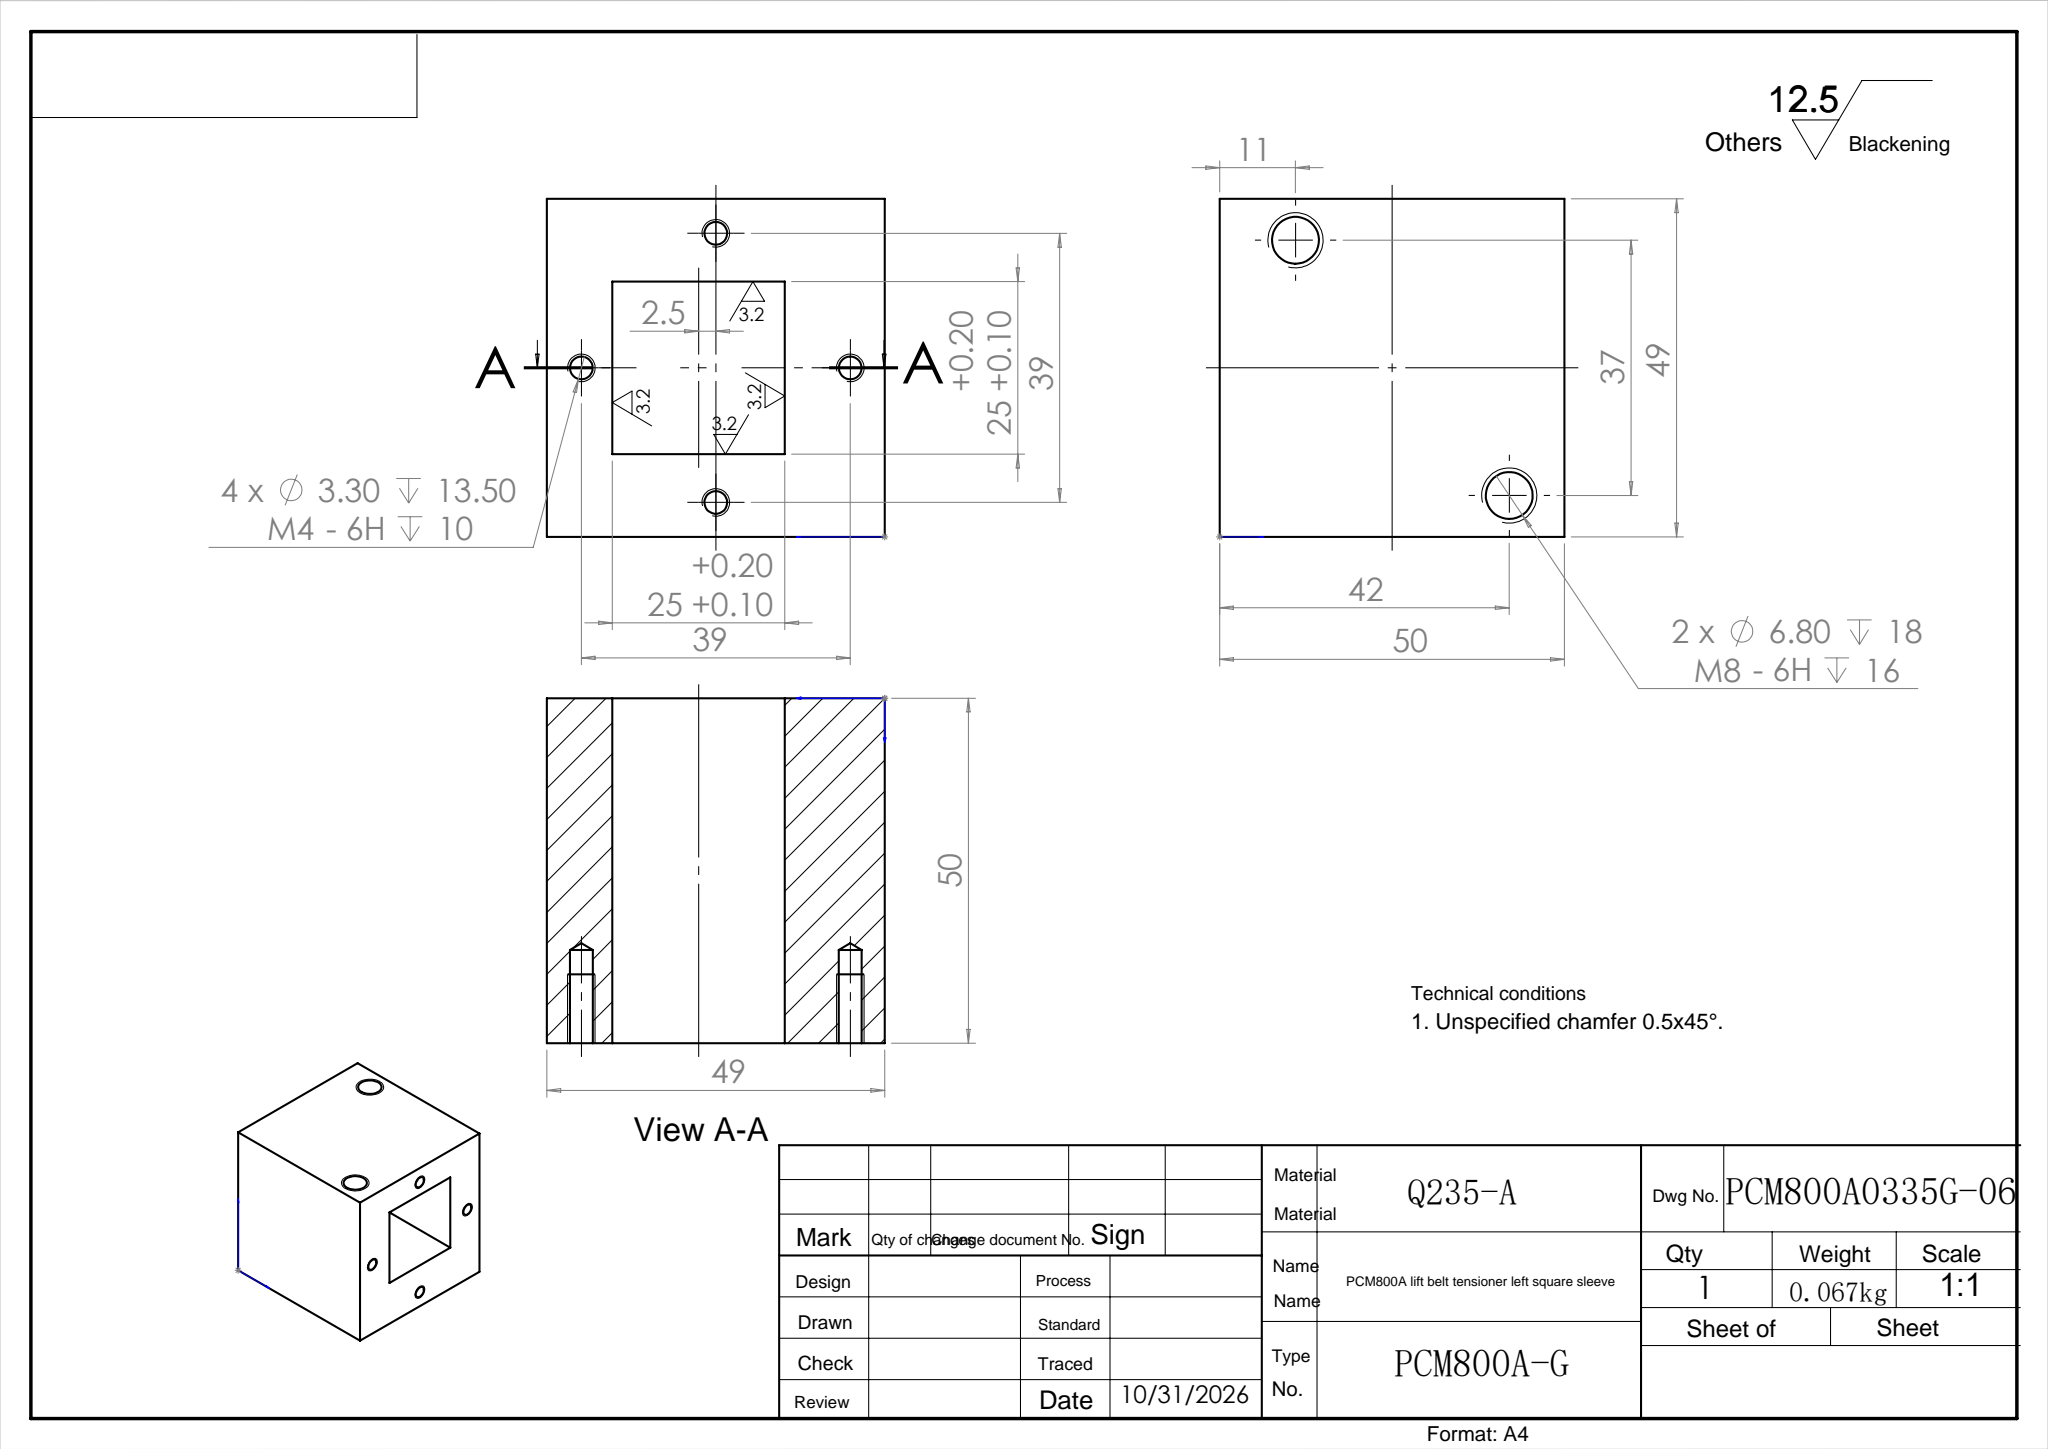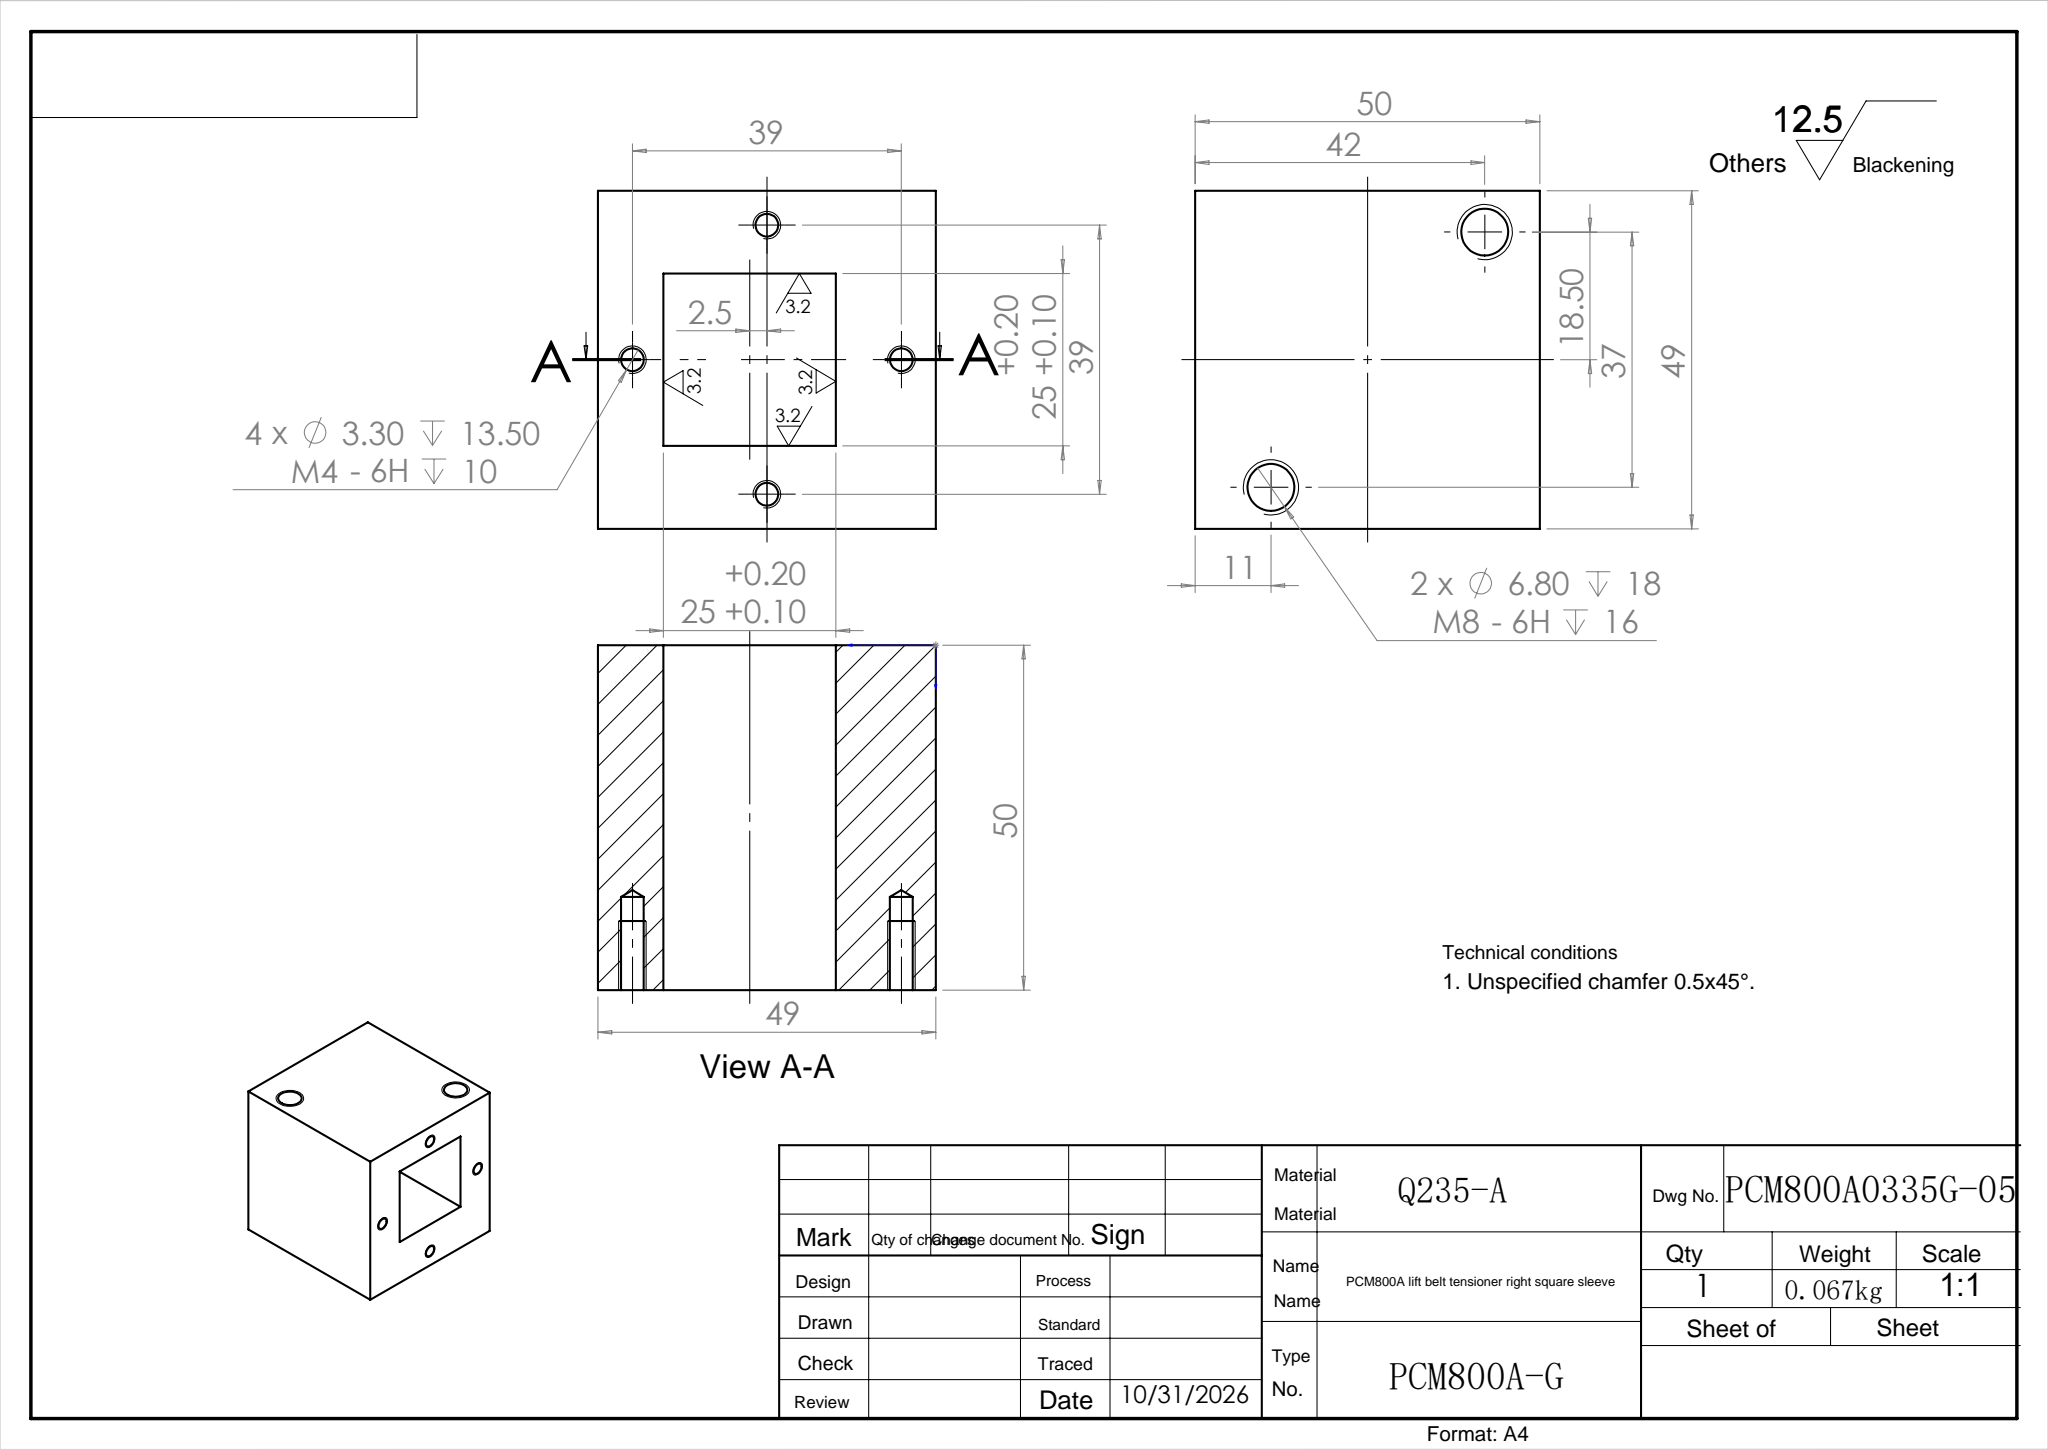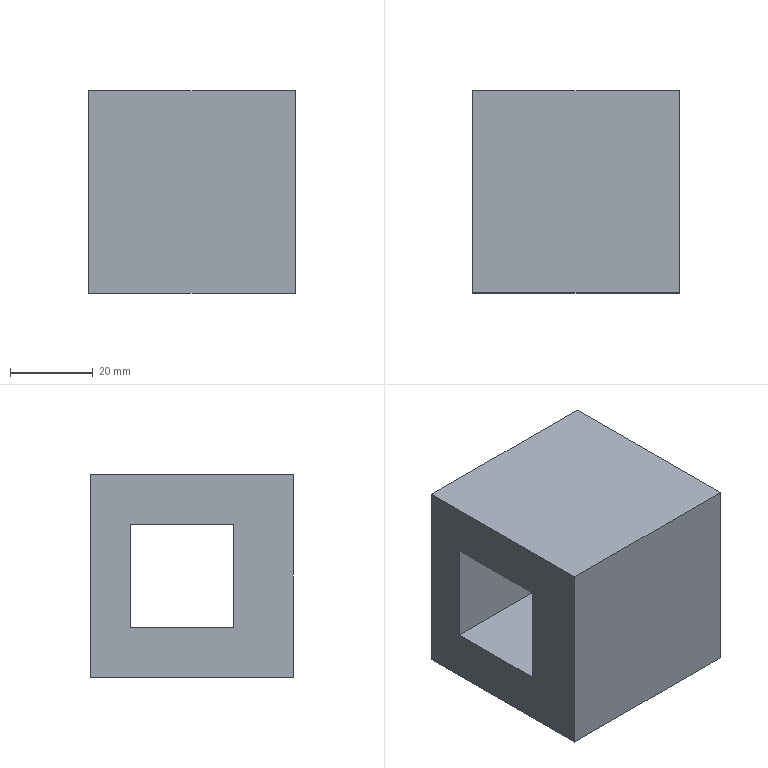Part | SolidWorks | features HoleWzd 2, Extrusion 1, ICE 1 | 1 solid | 34 faces | box 50 x 49 x 49 mm | volume 86970 mm3 | cylinder 12 | cone 12 | plane 10 | commonest cylinder face diameters 3.3 x8 6.8 x4
STEP:
#1=CARTESIAN_POINT('',(11.,31.,-9.4));
#2=VERTEX_POINT('',#1);
#3=CARTESIAN_POINT('',(11.,31.,-2.6));
#4=VERTEX_POINT('',#3);
#5=CARTESIAN_POINT('',(11.,31.,-6.));
#6=DIRECTION('',(0.,1.,0.));
#7=DIRECTION('',(0.,0.,1.));
#8=AXIS2_PLACEMENT_3D('',#5,#6,#7);
#9=CIRCLE('',#8,3.4);
#10=EDGE_CURVE('',#2,#4,#9,.T.);
#11=ORIENTED_EDGE('',*,*,#10,.F.);
#12=CARTESIAN_POINT('',(11.,49.,-9.4));
#13=VERTEX_POINT('',#12);
#14=CARTESIAN_POINT('',(11.,49.,-9.4));
#15=DIRECTION('',(0.,1.,0.));
#16=VECTOR('',#15,1000.);
#17=LINE('',#14,#16);
#18=EDGE_CURVE('',#2,#13,#17,.T.);
#19=ORIENTED_EDGE('',*,*,#18,.T.);
#20=CARTESIAN_POINT('',(11.,49.,-2.6));
#21=VERTEX_POINT('',#20);
#22=CARTESIAN_POINT('',(11.,49.,-6.));
#23=DIRECTION('',(0.,1.,0.));
#24=DIRECTION('',(0.,0.,1.));
#25=AXIS2_PLACEMENT_3D('',#22,#23,#24);
#26=CIRCLE('',#25,3.4);
#27=EDGE_CURVE('',#13,#21,#26,.T.);
#28=ORIENTED_EDGE('',*,*,#27,.T.);
#29=CARTESIAN_POINT('',(11.,49.,-2.6));
#30=DIRECTION('',(0.,1.,0.));
#31=VECTOR('',#30,1000.);
#32=LINE('',#29,#31);
#33=EDGE_CURVE('',#4,#21,#32,.T.);
#34=ORIENTED_EDGE('',*,*,#33,.F.);
#35=EDGE_LOOP('',(#11,#19,#28,#34));
#36=FACE_OUTER_BOUND('',#35,.T.);
#37=CARTESIAN_POINT('',(11.,49.,-6.));
#38=DIRECTION('',(0.,1.,0.));
#39=DIRECTION('',(0.,0.,1.));
#40=AXIS2_PLACEMENT_3D('',#37,#38,#39);
#41=CYLINDRICAL_SURFACE('',#40,3.4);
#42=ADVANCED_FACE('',(#36),#41,.F.);
#43=CARTESIAN_POINT('',(11.,28.957,-6.));
#44=VERTEX_POINT('',#43);
#45=CARTESIAN_POINT('',(11.,31.,-2.6));
#46=DIRECTION('',(0.,0.515,0.8572));
#47=VECTOR('',#46,1000.);
#48=LINE('',#45,#47);
#49=EDGE_CURVE('',#44,#4,#48,.T.);
#50=ORIENTED_EDGE('',*,*,#49,.F.);
#51=CARTESIAN_POINT('',(11.,31.,-9.4));
#52=DIRECTION('',(0.,0.515,-0.8572));
#53=VECTOR('',#52,1000.);
#54=LINE('',#51,#53);
#55=EDGE_CURVE('',#44,#2,#54,.T.);
#56=ORIENTED_EDGE('',*,*,#55,.T.);
#57=ORIENTED_EDGE('',*,*,#10,.T.);
#58=EDGE_LOOP('',(#50,#56,#57));
#59=FACE_OUTER_BOUND('',#58,.T.);
#60=CARTESIAN_POINT('',(11.,31.,-6.));
#61=DIRECTION('',(0.,1.,0.));
#62=DIRECTION('',(0.,0.,1.));
#63=AXIS2_PLACEMENT_3D('',#60,#61,#62);
#64=CONICAL_SURFACE('',#63,3.4,1.03);
#65=ADVANCED_FACE('',(#59),#64,.F.);
#66=CARTESIAN_POINT('',(42.,31.,-46.4));
#67=VERTEX_POINT('',#66);
#68=CARTESIAN_POINT('',(42.,31.,-39.6));
#69=VERTEX_POINT('',#68);
#70=CARTESIAN_POINT('',(42.,31.,-43.));
#71=DIRECTION('',(0.,1.,0.));
#72=DIRECTION('',(0.,0.,1.));
#73=AXIS2_PLACEMENT_3D('',#70,#71,#72);
#74=CIRCLE('',#73,3.4);
#75=EDGE_CURVE('',#67,#69,#74,.T.);
#76=ORIENTED_EDGE('',*,*,#75,.F.);
#77=CARTESIAN_POINT('',(42.,49.,-46.4));
#78=VERTEX_POINT('',#77);
#79=CARTESIAN_POINT('',(42.,49.,-46.4));
#80=DIRECTION('',(0.,1.,0.));
#81=VECTOR('',#80,1000.);
#82=LINE('',#79,#81);
#83=EDGE_CURVE('',#67,#78,#82,.T.);
#84=ORIENTED_EDGE('',*,*,#83,.T.);
#85=CARTESIAN_POINT('',(42.,49.,-39.6));
#86=VERTEX_POINT('',#85);
#87=CARTESIAN_POINT('',(42.,49.,-43.));
#88=DIRECTION('',(0.,1.,0.));
#89=DIRECTION('',(0.,0.,1.));
#90=AXIS2_PLACEMENT_3D('',#87,#88,#89);
#91=CIRCLE('',#90,3.4);
#92=EDGE_CURVE('',#78,#86,#91,.T.);
#93=ORIENTED_EDGE('',*,*,#92,.T.);
#94=CARTESIAN_POINT('',(42.,49.,-39.6));
#95=DIRECTION('',(0.,1.,0.));
#96=VECTOR('',#95,1000.);
#97=LINE('',#94,#96);
#98=EDGE_CURVE('',#69,#86,#97,.T.);
#99=ORIENTED_EDGE('',*,*,#98,.F.);
#100=EDGE_LOOP('',(#76,#84,#93,#99));
#101=FACE_OUTER_BOUND('',#100,.T.);
#102=CARTESIAN_POINT('',(42.,49.,-43.));
#103=DIRECTION('',(0.,1.,0.));
#104=DIRECTION('',(0.,0.,1.));
#105=AXIS2_PLACEMENT_3D('',#102,#103,#104);
#106=CYLINDRICAL_SURFACE('',#105,3.4);
#107=ADVANCED_FACE('',(#101),#106,.F.);
#108=CARTESIAN_POINT('',(42.,28.957,-43.));
#109=VERTEX_POINT('',#108);
#110=CARTESIAN_POINT('',(42.,31.,-39.6));
#111=DIRECTION('',(0.,0.515,0.8572));
#112=VECTOR('',#111,1000.);
#113=LINE('',#110,#112);
#114=EDGE_CURVE('',#109,#69,#113,.T.);
#115=ORIENTED_EDGE('',*,*,#114,.F.);
#116=CARTESIAN_POINT('',(42.,31.,-46.4));
#117=DIRECTION('',(0.,0.515,-0.8572));
#118=VECTOR('',#117,1000.);
#119=LINE('',#116,#118);
#120=EDGE_CURVE('',#109,#67,#119,.T.);
#121=ORIENTED_EDGE('',*,*,#120,.T.);
#122=ORIENTED_EDGE('',*,*,#75,.T.);
#123=EDGE_LOOP('',(#115,#121,#122));
#124=FACE_OUTER_BOUND('',#123,.T.);
#125=CARTESIAN_POINT('',(42.,31.,-43.));
#126=DIRECTION('',(0.,1.,0.));
#127=DIRECTION('',(0.,0.,1.));
#128=AXIS2_PLACEMENT_3D('',#125,#126,#127);
#129=CONICAL_SURFACE('',#128,3.4,1.03);
#130=ADVANCED_FACE('',(#124),#129,.F.);
#131=CARTESIAN_POINT('',(36.5,44.,-22.85));
#132=VERTEX_POINT('',#131);
#133=CARTESIAN_POINT('',(36.5,44.,-26.15));
#134=VERTEX_POINT('',#133);
#135=CARTESIAN_POINT('',(36.5,44.,-24.5));
#136=DIRECTION('',(1.,0.,0.));
#137=DIRECTION('',(0.,0.,-1.));
#138=AXIS2_PLACEMENT_3D('',#135,#136,#137);
#139=CIRCLE('',#138,1.65);
#140=EDGE_CURVE('',#132,#134,#139,.T.);
#141=ORIENTED_EDGE('',*,*,#140,.F.);
#142=CARTESIAN_POINT('',(50.,44.,-22.85));
#143=VERTEX_POINT('',#142);
#144=CARTESIAN_POINT('',(50.,44.,-22.85));
#145=DIRECTION('',(1.,0.,0.));
#146=VECTOR('',#145,1000.);
#147=LINE('',#144,#146);
#148=EDGE_CURVE('',#132,#143,#147,.T.);
#149=ORIENTED_EDGE('',*,*,#148,.T.);
#150=CARTESIAN_POINT('',(50.,44.,-26.15));
#151=VERTEX_POINT('',#150);
#152=CARTESIAN_POINT('',(50.,44.,-24.5));
#153=DIRECTION('',(1.,0.,0.));
#154=DIRECTION('',(0.,0.,-1.));
#155=AXIS2_PLACEMENT_3D('',#152,#153,#154);
#156=CIRCLE('',#155,1.65);
#157=EDGE_CURVE('',#143,#151,#156,.T.);
#158=ORIENTED_EDGE('',*,*,#157,.T.);
#159=CARTESIAN_POINT('',(50.,44.,-26.15));
#160=DIRECTION('',(1.,0.,0.));
#161=VECTOR('',#160,1000.);
#162=LINE('',#159,#161);
#163=EDGE_CURVE('',#134,#151,#162,.T.);
#164=ORIENTED_EDGE('',*,*,#163,.F.);
#165=EDGE_LOOP('',(#141,#149,#158,#164));
#166=FACE_OUTER_BOUND('',#165,.T.);
#167=CARTESIAN_POINT('',(50.,44.,-24.5));
#168=DIRECTION('',(1.,0.,0.));
#169=DIRECTION('',(0.,0.,-1.));
#170=AXIS2_PLACEMENT_3D('',#167,#168,#169);
#171=CYLINDRICAL_SURFACE('',#170,1.65);
#172=ADVANCED_FACE('',(#166),#171,.F.);
#173=CARTESIAN_POINT('',(35.509,44.,-24.5));
#174=VERTEX_POINT('',#173);
#175=CARTESIAN_POINT('',(36.5,44.,-26.15));
#176=DIRECTION('',(0.515,0.,-0.8572));
#177=VECTOR('',#176,1000.);
#178=LINE('',#175,#177);
#179=EDGE_CURVE('',#174,#134,#178,.T.);
#180=ORIENTED_EDGE('',*,*,#179,.F.);
#181=CARTESIAN_POINT('',(36.5,44.,-22.85));
#182=DIRECTION('',(0.515,0.,0.8572));
#183=VECTOR('',#182,1000.);
#184=LINE('',#181,#183);
#185=EDGE_CURVE('',#174,#132,#184,.T.);
#186=ORIENTED_EDGE('',*,*,#185,.T.);
#187=ORIENTED_EDGE('',*,*,#140,.T.);
#188=EDGE_LOOP('',(#180,#186,#187));
#189=FACE_OUTER_BOUND('',#188,.T.);
#190=CARTESIAN_POINT('',(36.5,44.,-24.5));
#191=DIRECTION('',(1.,0.,0.));
#192=DIRECTION('',(0.,0.,-1.));
#193=AXIS2_PLACEMENT_3D('',#190,#191,#192);
#194=CONICAL_SURFACE('',#193,1.65,1.03);
#195=ADVANCED_FACE('',(#189),#194,.F.);
#196=CARTESIAN_POINT('',(36.5,24.5,-3.35));
#197=VERTEX_POINT('',#196);
#198=CARTESIAN_POINT('',(36.5,24.5,-6.65));
#199=VERTEX_POINT('',#198);
#200=CARTESIAN_POINT('',(36.5,24.5,-5.));
#201=DIRECTION('',(1.,0.,0.));
#202=DIRECTION('',(0.,0.,-1.));
#203=AXIS2_PLACEMENT_3D('',#200,#201,#202);
#204=CIRCLE('',#203,1.65);
#205=EDGE_CURVE('',#197,#199,#204,.T.);
#206=ORIENTED_EDGE('',*,*,#205,.F.);
#207=CARTESIAN_POINT('',(50.,24.5,-3.35));
#208=VERTEX_POINT('',#207);
#209=CARTESIAN_POINT('',(50.,24.5,-3.35));
#210=DIRECTION('',(1.,0.,0.));
#211=VECTOR('',#210,1000.);
#212=LINE('',#209,#211);
#213=EDGE_CURVE('',#197,#208,#212,.T.);
#214=ORIENTED_EDGE('',*,*,#213,.T.);
#215=CARTESIAN_POINT('',(50.,24.5,-6.65));
#216=VERTEX_POINT('',#215);
#217=CARTESIAN_POINT('',(50.,24.5,-5.));
#218=DIRECTION('',(1.,0.,0.));
#219=DIRECTION('',(0.,0.,-1.));
#220=AXIS2_PLACEMENT_3D('',#217,#218,#219);
#221=CIRCLE('',#220,1.65);
#222=EDGE_CURVE('',#208,#216,#221,.T.);
#223=ORIENTED_EDGE('',*,*,#222,.T.);
#224=CARTESIAN_POINT('',(50.,24.5,-6.65));
#225=DIRECTION('',(1.,0.,0.));
#226=VECTOR('',#225,1000.);
#227=LINE('',#224,#226);
#228=EDGE_CURVE('',#199,#216,#227,.T.);
#229=ORIENTED_EDGE('',*,*,#228,.F.);
#230=EDGE_LOOP('',(#206,#214,#223,#229));
#231=FACE_OUTER_BOUND('',#230,.T.);
#232=CARTESIAN_POINT('',(50.,24.5,-5.));
#233=DIRECTION('',(1.,0.,0.));
#234=DIRECTION('',(0.,0.,-1.));
#235=AXIS2_PLACEMENT_3D('',#232,#233,#234);
#236=CYLINDRICAL_SURFACE('',#235,1.65);
#237=ADVANCED_FACE('',(#231),#236,.F.);
#238=CARTESIAN_POINT('',(35.509,24.5,-5.));
#239=VERTEX_POINT('',#238);
#240=CARTESIAN_POINT('',(36.5,24.5,-6.65));
#241=DIRECTION('',(0.515,0.,-0.8572));
#242=VECTOR('',#241,1000.);
#243=LINE('',#240,#242);
#244=EDGE_CURVE('',#239,#199,#243,.T.);
#245=ORIENTED_EDGE('',*,*,#244,.F.);
#246=CARTESIAN_POINT('',(36.5,24.5,-3.35));
#247=DIRECTION('',(0.515,0.,0.8572));
#248=VECTOR('',#247,1000.);
#249=LINE('',#246,#248);
#250=EDGE_CURVE('',#239,#197,#249,.T.);
#251=ORIENTED_EDGE('',*,*,#250,.T.);
#252=ORIENTED_EDGE('',*,*,#205,.T.);
#253=EDGE_LOOP('',(#245,#251,#252));
#254=FACE_OUTER_BOUND('',#253,.T.);
#255=CARTESIAN_POINT('',(36.5,24.5,-5.));
#256=DIRECTION('',(1.,0.,0.));
#257=DIRECTION('',(0.,0.,-1.));
#258=AXIS2_PLACEMENT_3D('',#255,#256,#257);
#259=CONICAL_SURFACE('',#258,1.65,1.03);
#260=ADVANCED_FACE('',(#254),#259,.F.);
#261=CARTESIAN_POINT('',(36.5,5.,-22.85));
#262=VERTEX_POINT('',#261);
#263=CARTESIAN_POINT('',(36.5,5.,-26.15));
#264=VERTEX_POINT('',#263);
#265=CARTESIAN_POINT('',(36.5,5.,-24.5));
#266=DIRECTION('',(1.,0.,0.));
#267=DIRECTION('',(0.,0.,-1.));
#268=AXIS2_PLACEMENT_3D('',#265,#266,#267);
#269=CIRCLE('',#268,1.65);
#270=EDGE_CURVE('',#262,#264,#269,.T.);
#271=ORIENTED_EDGE('',*,*,#270,.F.);
#272=CARTESIAN_POINT('',(50.,5.,-22.85));
#273=VERTEX_POINT('',#272);
#274=CARTESIAN_POINT('',(50.,5.,-22.85));
#275=DIRECTION('',(1.,0.,0.));
#276=VECTOR('',#275,1000.);
#277=LINE('',#274,#276);
#278=EDGE_CURVE('',#262,#273,#277,.T.);
#279=ORIENTED_EDGE('',*,*,#278,.T.);
#280=CARTESIAN_POINT('',(50.,5.,-26.15));
#281=VERTEX_POINT('',#280);
#282=CARTESIAN_POINT('',(50.,5.,-24.5));
#283=DIRECTION('',(1.,0.,0.));
#284=DIRECTION('',(0.,0.,-1.));
#285=AXIS2_PLACEMENT_3D('',#282,#283,#284);
#286=CIRCLE('',#285,1.65);
#287=EDGE_CURVE('',#273,#281,#286,.T.);
#288=ORIENTED_EDGE('',*,*,#287,.T.);
#289=CARTESIAN_POINT('',(50.,5.,-26.15));
#290=DIRECTION('',(1.,0.,0.));
#291=VECTOR('',#290,1000.);
#292=LINE('',#289,#291);
#293=EDGE_CURVE('',#264,#281,#292,.T.);
#294=ORIENTED_EDGE('',*,*,#293,.F.);
#295=EDGE_LOOP('',(#271,#279,#288,#294));
#296=FACE_OUTER_BOUND('',#295,.T.);
#297=CARTESIAN_POINT('',(50.,5.,-24.5));
#298=DIRECTION('',(1.,0.,0.));
#299=DIRECTION('',(0.,0.,-1.));
#300=AXIS2_PLACEMENT_3D('',#297,#298,#299);
#301=CYLINDRICAL_SURFACE('',#300,1.65);
#302=ADVANCED_FACE('',(#296),#301,.F.);
#303=CARTESIAN_POINT('',(35.509,5.,-24.5));
#304=VERTEX_POINT('',#303);
#305=CARTESIAN_POINT('',(36.5,5.,-26.15));
#306=DIRECTION('',(0.515,0.,-0.8572));
#307=VECTOR('',#306,1000.);
#308=LINE('',#305,#307);
#309=EDGE_CURVE('',#304,#264,#308,.T.);
#310=ORIENTED_EDGE('',*,*,#309,.F.);
#311=CARTESIAN_POINT('',(36.5,5.,-22.85));
#312=DIRECTION('',(0.515,0.,0.8572));
#313=VECTOR('',#312,1000.);
#314=LINE('',#311,#313);
#315=EDGE_CURVE('',#304,#262,#314,.T.);
#316=ORIENTED_EDGE('',*,*,#315,.T.);
#317=ORIENTED_EDGE('',*,*,#270,.T.);
#318=EDGE_LOOP('',(#310,#316,#317));
#319=FACE_OUTER_BOUND('',#318,.T.);
#320=CARTESIAN_POINT('',(36.5,5.,-24.5));
#321=DIRECTION('',(1.,0.,0.));
#322=DIRECTION('',(0.,0.,-1.));
#323=AXIS2_PLACEMENT_3D('',#320,#321,#322);
#324=CONICAL_SURFACE('',#323,1.65,1.03);
#325=ADVANCED_FACE('',(#319),#324,.F.);
#326=CARTESIAN_POINT('',(36.5,24.5,-42.35));
#327=VERTEX_POINT('',#326);
#328=CARTESIAN_POINT('',(36.5,24.5,-45.65));
#329=VERTEX_POINT('',#328);
#330=CARTESIAN_POINT('',(36.5,24.5,-44.));
#331=DIRECTION('',(1.,0.,0.));
#332=DIRECTION('',(0.,0.,-1.));
#333=AXIS2_PLACEMENT_3D('',#330,#331,#332);
#334=CIRCLE('',#333,1.65);
#335=EDGE_CURVE('',#327,#329,#334,.T.);
#336=ORIENTED_EDGE('',*,*,#335,.F.);
#337=CARTESIAN_POINT('',(50.,24.5,-42.35));
#338=VERTEX_POINT('',#337);
#339=CARTESIAN_POINT('',(50.,24.5,-42.35));
#340=DIRECTION('',(1.,0.,0.));
#341=VECTOR('',#340,1000.);
#342=LINE('',#339,#341);
#343=EDGE_CURVE('',#327,#338,#342,.T.);
#344=ORIENTED_EDGE('',*,*,#343,.T.);
#345=CARTESIAN_POINT('',(50.,24.5,-45.65));
#346=VERTEX_POINT('',#345);
#347=CARTESIAN_POINT('',(50.,24.5,-44.));
#348=DIRECTION('',(1.,0.,0.));
#349=DIRECTION('',(0.,0.,-1.));
#350=AXIS2_PLACEMENT_3D('',#347,#348,#349);
#351=CIRCLE('',#350,1.65);
#352=EDGE_CURVE('',#338,#346,#351,.T.);
#353=ORIENTED_EDGE('',*,*,#352,.T.);
#354=CARTESIAN_POINT('',(50.,24.5,-45.65));
#355=DIRECTION('',(1.,0.,0.));
#356=VECTOR('',#355,1000.);
#357=LINE('',#354,#356);
#358=EDGE_CURVE('',#329,#346,#357,.T.);
#359=ORIENTED_EDGE('',*,*,#358,.F.);
#360=EDGE_LOOP('',(#336,#344,#353,#359));
#361=FACE_OUTER_BOUND('',#360,.T.);
#362=CARTESIAN_POINT('',(50.,24.5,-44.));
#363=DIRECTION('',(1.,0.,0.));
#364=DIRECTION('',(0.,0.,-1.));
#365=AXIS2_PLACEMENT_3D('',#362,#363,#364);
#366=CYLINDRICAL_SURFACE('',#365,1.65);
#367=ADVANCED_FACE('',(#361),#366,.F.);
#368=CARTESIAN_POINT('',(35.509,24.5,-44.));
#369=VERTEX_POINT('',#368);
#370=CARTESIAN_POINT('',(36.5,24.5,-45.65));
#371=DIRECTION('',(0.515,0.,-0.8572));
#372=VECTOR('',#371,1000.);
#373=LINE('',#370,#372);
#374=EDGE_CURVE('',#369,#329,#373,.T.);
#375=ORIENTED_EDGE('',*,*,#374,.F.);
#376=CARTESIAN_POINT('',(36.5,24.5,-42.35));
#377=DIRECTION('',(0.515,0.,0.8572));
#378=VECTOR('',#377,1000.);
#379=LINE('',#376,#378);
#380=EDGE_CURVE('',#369,#327,#379,.T.);
#381=ORIENTED_EDGE('',*,*,#380,.T.);
#382=ORIENTED_EDGE('',*,*,#335,.T.);
#383=EDGE_LOOP('',(#375,#381,#382));
#384=FACE_OUTER_BOUND('',#383,.T.);
#385=CARTESIAN_POINT('',(36.5,24.5,-44.));
#386=DIRECTION('',(1.,0.,0.));
#387=DIRECTION('',(0.,0.,-1.));
#388=AXIS2_PLACEMENT_3D('',#385,#386,#387);
#389=CONICAL_SURFACE('',#388,1.65,1.03);
#390=ADVANCED_FACE('',(#384),#389,.F.);
#391=CARTESIAN_POINT('',(0.,49.,0.));
#392=VERTEX_POINT('',#391);
#393=CARTESIAN_POINT('',(0.,0.,0.));
#394=VERTEX_POINT('',#393);
#395=CARTESIAN_POINT('',(0.,0.,0.));
#396=DIRECTION('',(0.,-1.,0.));
#397=VECTOR('',#396,1000.);
#398=LINE('',#395,#397);
#399=EDGE_CURVE('',#392,#394,#398,.T.);
#400=ORIENTED_EDGE('',*,*,#399,.T.);
#401=CARTESIAN_POINT('',(50.,0.,0.));
#402=VERTEX_POINT('',#401);
#403=CARTESIAN_POINT('',(50.,0.,0.));
#404=DIRECTION('',(-1.,0.,0.));
#405=VECTOR('',#404,1000.);
#406=LINE('',#403,#405);
#407=EDGE_CURVE('',#402,#394,#406,.T.);
#408=ORIENTED_EDGE('',*,*,#407,.F.);
#409=CARTESIAN_POINT('',(50.,49.,0.));
#410=VERTEX_POINT('',#409);
#411=CARTESIAN_POINT('',(50.,0.,0.));
#412=DIRECTION('',(0.,-1.,0.));
#413=VECTOR('',#412,1000.);
#414=LINE('',#411,#413);
#415=EDGE_CURVE('',#410,#402,#414,.T.);
#416=ORIENTED_EDGE('',*,*,#415,.F.);
#417=CARTESIAN_POINT('',(50.,49.,0.));
#418=DIRECTION('',(-1.,0.,0.));
#419=VECTOR('',#418,1000.);
#420=LINE('',#417,#419);
#421=EDGE_CURVE('',#410,#392,#420,.T.);
#422=ORIENTED_EDGE('',*,*,#421,.T.);
#423=EDGE_LOOP('',(#400,#408,#416,#422));
#424=FACE_OUTER_BOUND('',#423,.T.);
#425=CARTESIAN_POINT('',(50.,0.,0.));
#426=DIRECTION('',(0.,0.,-1.));
#427=DIRECTION('',(0.,1.,0.));
#428=AXIS2_PLACEMENT_3D('',#425,#426,#427);
#429=PLANE('',#428);
#430=ADVANCED_FACE('',(#424),#429,.F.);
#431=CARTESIAN_POINT('',(0.,0.,-49.));
#432=VERTEX_POINT('',#431);
#433=CARTESIAN_POINT('',(0.,0.,0.));
#434=DIRECTION('',(0.,0.,-1.));
#435=VECTOR('',#434,1000.);
#436=LINE('',#433,#435);
#437=EDGE_CURVE('',#394,#432,#436,.T.);
#438=ORIENTED_EDGE('',*,*,#437,.T.);
#439=CARTESIAN_POINT('',(50.,0.,-49.));
#440=VERTEX_POINT('',#439);
#441=CARTESIAN_POINT('',(50.,0.,-49.));
#442=DIRECTION('',(-1.,0.,0.));
#443=VECTOR('',#442,1000.);
#444=LINE('',#441,#443);
#445=EDGE_CURVE('',#440,#432,#444,.T.);
#446=ORIENTED_EDGE('',*,*,#445,.F.);
#447=CARTESIAN_POINT('',(50.,0.,0.));
#448=DIRECTION('',(0.,0.,-1.));
#449=VECTOR('',#448,1000.);
#450=LINE('',#447,#449);
#451=EDGE_CURVE('',#402,#440,#450,.T.);
#452=ORIENTED_EDGE('',*,*,#451,.F.);
#453=ORIENTED_EDGE('',*,*,#407,.T.);
#454=EDGE_LOOP('',(#438,#446,#452,#453));
#455=FACE_OUTER_BOUND('',#454,.T.);
#456=CARTESIAN_POINT('',(50.,0.,0.));
#457=DIRECTION('',(0.,1.,0.));
#458=DIRECTION('',(0.,0.,1.));
#459=AXIS2_PLACEMENT_3D('',#456,#457,#458);
#460=PLANE('',#459);
#461=ADVANCED_FACE('',(#455),#460,.F.);
#462=CARTESIAN_POINT('',(0.,49.,-49.));
#463=VERTEX_POINT('',#462);
#464=CARTESIAN_POINT('',(0.,0.,-49.));
#465=DIRECTION('',(0.,1.,0.));
#466=VECTOR('',#465,1000.);
#467=LINE('',#464,#466);
#468=EDGE_CURVE('',#432,#463,#467,.T.);
#469=ORIENTED_EDGE('',*,*,#468,.T.);
#470=CARTESIAN_POINT('',(50.,49.,-49.));
#471=VERTEX_POINT('',#470);
#472=CARTESIAN_POINT('',(50.,49.,-49.));
#473=DIRECTION('',(-1.,0.,0.));
#474=VECTOR('',#473,1000.);
#475=LINE('',#472,#474);
#476=EDGE_CURVE('',#471,#463,#475,.T.);
#477=ORIENTED_EDGE('',*,*,#476,.F.);
#478=CARTESIAN_POINT('',(50.,0.,-49.));
#479=DIRECTION('',(0.,1.,0.));
#480=VECTOR('',#479,1000.);
#481=LINE('',#478,#480);
#482=EDGE_CURVE('',#440,#471,#481,.T.);
#483=ORIENTED_EDGE('',*,*,#482,.F.);
#484=ORIENTED_EDGE('',*,*,#445,.T.);
#485=EDGE_LOOP('',(#469,#477,#483,#484));
#486=FACE_OUTER_BOUND('',#485,.T.);
#487=CARTESIAN_POINT('',(50.,0.,-49.));
#488=DIRECTION('',(0.,0.,1.));
#489=DIRECTION('',(0.,-1.,0.));
#490=AXIS2_PLACEMENT_3D('',#487,#488,#489);
#491=PLANE('',#490);
#492=ADVANCED_FACE('',(#486),#491,.F.);
#493=CARTESIAN_POINT('',(11.,49.,-6.));
#494=DIRECTION('',(0.,1.,0.));
#495=DIRECTION('',(0.,0.,1.));
#496=AXIS2_PLACEMENT_3D('',#493,#494,#495);
#497=CIRCLE('',#496,3.4);
#498=EDGE_CURVE('',#21,#13,#497,.T.);
#499=ORIENTED_EDGE('',*,*,#498,.F.);
#500=ORIENTED_EDGE('',*,*,#27,.F.);
#501=EDGE_LOOP('',(#499,#500));
#502=FACE_BOUND('',#501,.T.);
#503=CARTESIAN_POINT('',(42.,49.,-43.));
#504=DIRECTION('',(0.,1.,0.));
#505=DIRECTION('',(0.,0.,1.));
#506=AXIS2_PLACEMENT_3D('',#503,#504,#505);
#507=CIRCLE('',#506,3.4);
#508=EDGE_CURVE('',#86,#78,#507,.T.);
#509=ORIENTED_EDGE('',*,*,#508,.F.);
#510=ORIENTED_EDGE('',*,*,#92,.F.);
#511=EDGE_LOOP('',(#509,#510));
#512=FACE_BOUND('',#511,.T.);
#513=CARTESIAN_POINT('',(0.,49.,0.));
#514=DIRECTION('',(0.,0.,1.));
#515=VECTOR('',#514,1000.);
#516=LINE('',#513,#515);
#517=EDGE_CURVE('',#463,#392,#516,.T.);
#518=ORIENTED_EDGE('',*,*,#517,.T.);
#519=ORIENTED_EDGE('',*,*,#421,.F.);
#520=CARTESIAN_POINT('',(50.,49.,0.));
#521=DIRECTION('',(0.,0.,1.));
#522=VECTOR('',#521,1000.);
#523=LINE('',#520,#522);
#524=EDGE_CURVE('',#471,#410,#523,.T.);
#525=ORIENTED_EDGE('',*,*,#524,.F.);
#526=ORIENTED_EDGE('',*,*,#476,.T.);
#527=EDGE_LOOP('',(#518,#519,#525,#526));
#528=FACE_OUTER_BOUND('',#527,.T.);
#529=CARTESIAN_POINT('',(50.,49.,0.));
#530=DIRECTION('',(0.,-1.,0.));
#531=DIRECTION('',(0.,0.,-1.));
#532=AXIS2_PLACEMENT_3D('',#529,#530,#531);
#533=PLANE('',#532);
#534=ADVANCED_FACE('',(#502,#512,#528),#533,.F.);
#535=CARTESIAN_POINT('',(50.,44.,-24.5));
#536=DIRECTION('',(1.,0.,0.));
#537=DIRECTION('',(0.,0.,-1.));
#538=AXIS2_PLACEMENT_3D('',#535,#536,#537);
#539=CIRCLE('',#538,1.65);
#540=EDGE_CURVE('',#151,#143,#539,.T.);
#541=ORIENTED_EDGE('',*,*,#540,.F.);
#542=ORIENTED_EDGE('',*,*,#157,.F.);
#543=EDGE_LOOP('',(#541,#542));
#544=FACE_BOUND('',#543,.T.);
#545=CARTESIAN_POINT('',(50.,24.5,-5.));
#546=DIRECTION('',(1.,0.,0.));
#547=DIRECTION('',(0.,0.,-1.));
#548=AXIS2_PLACEMENT_3D('',#545,#546,#547);
#549=CIRCLE('',#548,1.65);
#550=EDGE_CURVE('',#216,#208,#549,.T.);
#551=ORIENTED_EDGE('',*,*,#550,.F.);
#552=ORIENTED_EDGE('',*,*,#222,.F.);
#553=EDGE_LOOP('',(#551,#552));
#554=FACE_BOUND('',#553,.T.);
#555=CARTESIAN_POINT('',(50.,5.,-24.5));
#556=DIRECTION('',(1.,0.,0.));
#557=DIRECTION('',(0.,0.,-1.));
#558=AXIS2_PLACEMENT_3D('',#555,#556,#557);
#559=CIRCLE('',#558,1.65);
#560=EDGE_CURVE('',#281,#273,#559,.T.);
#561=ORIENTED_EDGE('',*,*,#560,.F.);
#562=ORIENTED_EDGE('',*,*,#287,.F.);
#563=EDGE_LOOP('',(#561,#562));
#564=FACE_BOUND('',#563,.T.);
#565=CARTESIAN_POINT('',(50.,24.5,-44.));
#566=DIRECTION('',(1.,0.,0.));
#567=DIRECTION('',(0.,0.,-1.));
#568=AXIS2_PLACEMENT_3D('',#565,#566,#567);
#569=CIRCLE('',#568,1.65);
#570=EDGE_CURVE('',#346,#338,#569,.T.);
#571=ORIENTED_EDGE('',*,*,#570,.F.);
#572=ORIENTED_EDGE('',*,*,#352,.F.);
#573=EDGE_LOOP('',(#571,#572));
#574=FACE_BOUND('',#573,.T.);
#575=CARTESIAN_POINT('',(50.,14.5,-12.));
#576=VERTEX_POINT('',#575);
#577=CARTESIAN_POINT('',(50.,14.5,-37.));
#578=VERTEX_POINT('',#577);
#579=CARTESIAN_POINT('',(50.,14.5,-12.));
#580=DIRECTION('',(0.,0.,-1.));
#581=VECTOR('',#580,1000.);
#582=LINE('',#579,#581);
#583=EDGE_CURVE('',#576,#578,#582,.T.);
#584=ORIENTED_EDGE('',*,*,#583,.F.);
#585=CARTESIAN_POINT('',(50.,39.5,-12.));
#586=VERTEX_POINT('',#585);
#587=CARTESIAN_POINT('',(50.,39.5,-12.));
#588=DIRECTION('',(0.,-1.,0.));
#589=VECTOR('',#588,1000.);
#590=LINE('',#587,#589);
#591=EDGE_CURVE('',#586,#576,#590,.T.);
#592=ORIENTED_EDGE('',*,*,#591,.F.);
#593=CARTESIAN_POINT('',(50.,39.5,-37.));
#594=VERTEX_POINT('',#593);
#595=CARTESIAN_POINT('',(50.,39.5,-12.));
#596=DIRECTION('',(0.,0.,1.));
#597=VECTOR('',#596,1000.);
#598=LINE('',#595,#597);
#599=EDGE_CURVE('',#594,#586,#598,.T.);
#600=ORIENTED_EDGE('',*,*,#599,.F.);
#601=CARTESIAN_POINT('',(50.,39.5,-37.));
#602=DIRECTION('',(0.,1.,0.));
#603=VECTOR('',#602,1000.);
#604=LINE('',#601,#603);
#605=EDGE_CURVE('',#578,#594,#604,.T.);
#606=ORIENTED_EDGE('',*,*,#605,.F.);
#607=EDGE_LOOP('',(#584,#592,#600,#606));
#608=FACE_BOUND('',#607,.T.);
#609=ORIENTED_EDGE('',*,*,#415,.T.);
#610=ORIENTED_EDGE('',*,*,#451,.T.);
#611=ORIENTED_EDGE('',*,*,#482,.T.);
#612=ORIENTED_EDGE('',*,*,#524,.T.);
#613=EDGE_LOOP('',(#609,#610,#611,#612));
#614=FACE_OUTER_BOUND('',#613,.T.);
#615=CARTESIAN_POINT('',(50.,49.,0.));
#616=DIRECTION('',(-1.,0.,0.));
#617=DIRECTION('',(0.,0.,1.));
#618=AXIS2_PLACEMENT_3D('',#615,#616,#617);
#619=PLANE('',#618);
#620=ADVANCED_FACE('',(#544,#554,#564,#574,#608,#614),#619,.F.);
#621=CARTESIAN_POINT('',(0.,39.5,-12.));
#622=VERTEX_POINT('',#621);
#623=CARTESIAN_POINT('',(0.,14.5,-12.));
#624=VERTEX_POINT('',#623);
#625=CARTESIAN_POINT('',(0.,39.5,-12.));
#626=DIRECTION('',(0.,-1.,0.));
#627=VECTOR('',#626,1000.);
#628=LINE('',#625,#627);
#629=EDGE_CURVE('',#622,#624,#628,.T.);
#630=ORIENTED_EDGE('',*,*,#629,.T.);
#631=CARTESIAN_POINT('',(0.,14.5,-37.));
#632=VERTEX_POINT('',#631);
#633=CARTESIAN_POINT('',(0.,14.5,-12.));
#634=DIRECTION('',(0.,0.,-1.));
#635=VECTOR('',#634,1000.);
#636=LINE('',#633,#635);
#637=EDGE_CURVE('',#624,#632,#636,.T.);
#638=ORIENTED_EDGE('',*,*,#637,.T.);
#639=CARTESIAN_POINT('',(0.,39.5,-37.));
#640=VERTEX_POINT('',#639);
#641=CARTESIAN_POINT('',(0.,39.5,-37.));
#642=DIRECTION('',(0.,1.,0.));
#643=VECTOR('',#642,1000.);
#644=LINE('',#641,#643);
#645=EDGE_CURVE('',#632,#640,#644,.T.);
#646=ORIENTED_EDGE('',*,*,#645,.T.);
#647=CARTESIAN_POINT('',(0.,39.5,-12.));
#648=DIRECTION('',(0.,0.,1.));
#649=VECTOR('',#648,1000.);
#650=LINE('',#647,#649);
#651=EDGE_CURVE('',#640,#622,#650,.T.);
#652=ORIENTED_EDGE('',*,*,#651,.T.);
#653=EDGE_LOOP('',(#630,#638,#646,#652));
#654=FACE_BOUND('',#653,.T.);
#655=ORIENTED_EDGE('',*,*,#399,.F.);
#656=ORIENTED_EDGE('',*,*,#517,.F.);
#657=ORIENTED_EDGE('',*,*,#468,.F.);
#658=ORIENTED_EDGE('',*,*,#437,.F.);
#659=EDGE_LOOP('',(#655,#656,#657,#658));
#660=FACE_OUTER_BOUND('',#659,.T.);
#661=CARTESIAN_POINT('',(0.,49.,0.));
#662=DIRECTION('',(-1.,0.,0.));
#663=DIRECTION('',(0.,0.,1.));
#664=AXIS2_PLACEMENT_3D('',#661,#662,#663);
#665=PLANE('',#664);
#666=ADVANCED_FACE('',(#654,#660),#665,.T.);
#667=ORIENTED_EDGE('',*,*,#591,.T.);
#668=CARTESIAN_POINT('',(0.,14.5,-12.));
#669=DIRECTION('',(1.,0.,0.));
#670=VECTOR('',#669,1000.);
#671=LINE('',#668,#670);
#672=EDGE_CURVE('',#624,#576,#671,.T.);
#673=ORIENTED_EDGE('',*,*,#672,.F.);
#674=ORIENTED_EDGE('',*,*,#629,.F.);
#675=CARTESIAN_POINT('',(0.,39.5,-12.));
#676=DIRECTION('',(1.,0.,0.));
#677=VECTOR('',#676,1000.);
#678=LINE('',#675,#677);
#679=EDGE_CURVE('',#622,#586,#678,.T.);
#680=ORIENTED_EDGE('',*,*,#679,.T.);
#681=EDGE_LOOP('',(#667,#673,#674,#680));
#682=FACE_OUTER_BOUND('',#681,.T.);
#683=CARTESIAN_POINT('',(0.,39.5,-12.));
#684=DIRECTION('',(0.,0.,1.));
#685=DIRECTION('',(0.,-1.,0.));
#686=AXIS2_PLACEMENT_3D('',#683,#684,#685);
#687=PLANE('',#686);
#688=ADVANCED_FACE('',(#682),#687,.F.);
#689=ORIENTED_EDGE('',*,*,#599,.T.);
#690=ORIENTED_EDGE('',*,*,#679,.F.);
#691=ORIENTED_EDGE('',*,*,#651,.F.);
#692=CARTESIAN_POINT('',(0.,39.5,-37.));
#693=DIRECTION('',(1.,0.,0.));
#694=VECTOR('',#693,1000.);
#695=LINE('',#692,#694);
#696=EDGE_CURVE('',#640,#594,#695,.T.);
#697=ORIENTED_EDGE('',*,*,#696,.T.);
#698=EDGE_LOOP('',(#689,#690,#691,#697));
#699=FACE_OUTER_BOUND('',#698,.T.);
#700=CARTESIAN_POINT('',(0.,39.5,-12.));
#701=DIRECTION('',(0.,1.,0.));
#702=DIRECTION('',(0.,0.,1.));
#703=AXIS2_PLACEMENT_3D('',#700,#701,#702);
#704=PLANE('',#703);
#705=ADVANCED_FACE('',(#699),#704,.F.);
#706=ORIENTED_EDGE('',*,*,#605,.T.);
#707=ORIENTED_EDGE('',*,*,#696,.F.);
#708=ORIENTED_EDGE('',*,*,#645,.F.);
#709=CARTESIAN_POINT('',(0.,14.5,-37.));
#710=DIRECTION('',(1.,0.,0.));
#711=VECTOR('',#710,1000.);
#712=LINE('',#709,#711);
#713=EDGE_CURVE('',#632,#578,#712,.T.);
#714=ORIENTED_EDGE('',*,*,#713,.T.);
#715=EDGE_LOOP('',(#706,#707,#708,#714));
#716=FACE_OUTER_BOUND('',#715,.T.);
#717=CARTESIAN_POINT('',(0.,39.5,-37.));
#718=DIRECTION('',(0.,0.,-1.));
#719=DIRECTION('',(-1.,0.,0.));
#720=AXIS2_PLACEMENT_3D('',#717,#718,#719);
#721=PLANE('',#720);
#722=ADVANCED_FACE('',(#716),#721,.F.);
#723=ORIENTED_EDGE('',*,*,#583,.T.);
#724=ORIENTED_EDGE('',*,*,#713,.F.);
#725=ORIENTED_EDGE('',*,*,#637,.F.);
#726=ORIENTED_EDGE('',*,*,#672,.T.);
#727=EDGE_LOOP('',(#723,#724,#725,#726));
#728=FACE_OUTER_BOUND('',#727,.T.);
#729=CARTESIAN_POINT('',(0.,14.5,-12.));
#730=DIRECTION('',(0.,-1.,0.));
#731=DIRECTION('',(0.,0.,-1.));
#732=AXIS2_PLACEMENT_3D('',#729,#730,#731);
#733=PLANE('',#732);
#734=ADVANCED_FACE('',(#728),#733,.F.);
#735=ORIENTED_EDGE('',*,*,#380,.F.);
#736=ORIENTED_EDGE('',*,*,#374,.T.);
#737=CARTESIAN_POINT('',(36.5,24.5,-44.));
#738=DIRECTION('',(1.,0.,0.));
#739=DIRECTION('',(0.,0.,-1.));
#740=AXIS2_PLACEMENT_3D('',#737,#738,#739);
#741=CIRCLE('',#740,1.65);
#742=EDGE_CURVE('',#329,#327,#741,.T.);
#743=ORIENTED_EDGE('',*,*,#742,.T.);
#744=EDGE_LOOP('',(#735,#736,#743));
#745=FACE_OUTER_BOUND('',#744,.T.);
#746=CARTESIAN_POINT('',(36.5,24.5,-44.));
#747=DIRECTION('',(1.,0.,0.));
#748=DIRECTION('',(0.,0.,-1.));
#749=AXIS2_PLACEMENT_3D('',#746,#747,#748);
#750=CONICAL_SURFACE('',#749,1.65,1.03);
#751=ADVANCED_FACE('',(#745),#750,.F.);
#752=ORIENTED_EDGE('',*,*,#343,.F.);
#753=ORIENTED_EDGE('',*,*,#742,.F.);
#754=ORIENTED_EDGE('',*,*,#358,.T.);
#755=ORIENTED_EDGE('',*,*,#570,.T.);
#756=EDGE_LOOP('',(#752,#753,#754,#755));
#757=FACE_OUTER_BOUND('',#756,.T.);
#758=CARTESIAN_POINT('',(50.,24.5,-44.));
#759=DIRECTION('',(1.,0.,0.));
#760=DIRECTION('',(0.,0.,-1.));
#761=AXIS2_PLACEMENT_3D('',#758,#759,#760);
#762=CYLINDRICAL_SURFACE('',#761,1.65);
#763=ADVANCED_FACE('',(#757),#762,.F.);
#764=ORIENTED_EDGE('',*,*,#315,.F.);
#765=ORIENTED_EDGE('',*,*,#309,.T.);
#766=CARTESIAN_POINT('',(36.5,5.,-24.5));
#767=DIRECTION('',(1.,0.,0.));
#768=DIRECTION('',(0.,0.,-1.));
#769=AXIS2_PLACEMENT_3D('',#766,#767,#768);
#770=CIRCLE('',#769,1.65);
#771=EDGE_CURVE('',#264,#262,#770,.T.);
#772=ORIENTED_EDGE('',*,*,#771,.T.);
#773=EDGE_LOOP('',(#764,#765,#772));
#774=FACE_OUTER_BOUND('',#773,.T.);
#775=CARTESIAN_POINT('',(36.5,5.,-24.5));
#776=DIRECTION('',(1.,0.,0.));
#777=DIRECTION('',(0.,0.,-1.));
#778=AXIS2_PLACEMENT_3D('',#775,#776,#777);
#779=CONICAL_SURFACE('',#778,1.65,1.03);
#780=ADVANCED_FACE('',(#774),#779,.F.);
#781=ORIENTED_EDGE('',*,*,#278,.F.);
#782=ORIENTED_EDGE('',*,*,#771,.F.);
#783=ORIENTED_EDGE('',*,*,#293,.T.);
#784=ORIENTED_EDGE('',*,*,#560,.T.);
#785=EDGE_LOOP('',(#781,#782,#783,#784));
#786=FACE_OUTER_BOUND('',#785,.T.);
#787=CARTESIAN_POINT('',(50.,5.,-24.5));
#788=DIRECTION('',(1.,0.,0.));
#789=DIRECTION('',(0.,0.,-1.));
#790=AXIS2_PLACEMENT_3D('',#787,#788,#789);
#791=CYLINDRICAL_SURFACE('',#790,1.65);
#792=ADVANCED_FACE('',(#786),#791,.F.);
#793=ORIENTED_EDGE('',*,*,#250,.F.);
#794=ORIENTED_EDGE('',*,*,#244,.T.);
#795=CARTESIAN_POINT('',(36.5,24.5,-5.));
#796=DIRECTION('',(1.,0.,0.));
#797=DIRECTION('',(0.,0.,-1.));
#798=AXIS2_PLACEMENT_3D('',#795,#796,#797);
#799=CIRCLE('',#798,1.65);
#800=EDGE_CURVE('',#199,#197,#799,.T.);
#801=ORIENTED_EDGE('',*,*,#800,.T.);
#802=EDGE_LOOP('',(#793,#794,#801));
#803=FACE_OUTER_BOUND('',#802,.T.);
#804=CARTESIAN_POINT('',(36.5,24.5,-5.));
#805=DIRECTION('',(1.,0.,0.));
#806=DIRECTION('',(0.,0.,-1.));
#807=AXIS2_PLACEMENT_3D('',#804,#805,#806);
#808=CONICAL_SURFACE('',#807,1.65,1.03);
#809=ADVANCED_FACE('',(#803),#808,.F.);
#810=ORIENTED_EDGE('',*,*,#213,.F.);
#811=ORIENTED_EDGE('',*,*,#800,.F.);
#812=ORIENTED_EDGE('',*,*,#228,.T.);
#813=ORIENTED_EDGE('',*,*,#550,.T.);
#814=EDGE_LOOP('',(#810,#811,#812,#813));
#815=FACE_OUTER_BOUND('',#814,.T.);
#816=CARTESIAN_POINT('',(50.,24.5,-5.));
#817=DIRECTION('',(1.,0.,0.));
#818=DIRECTION('',(0.,0.,-1.));
#819=AXIS2_PLACEMENT_3D('',#816,#817,#818);
#820=CYLINDRICAL_SURFACE('',#819,1.65);
#821=ADVANCED_FACE('',(#815),#820,.F.);
#822=ORIENTED_EDGE('',*,*,#185,.F.);
#823=ORIENTED_EDGE('',*,*,#179,.T.);
#824=CARTESIAN_POINT('',(36.5,44.,-24.5));
#825=DIRECTION('',(1.,0.,0.));
#826=DIRECTION('',(0.,0.,-1.));
#827=AXIS2_PLACEMENT_3D('',#824,#825,#826);
#828=CIRCLE('',#827,1.65);
#829=EDGE_CURVE('',#134,#132,#828,.T.);
#830=ORIENTED_EDGE('',*,*,#829,.T.);
#831=EDGE_LOOP('',(#822,#823,#830));
#832=FACE_OUTER_BOUND('',#831,.T.);
#833=CARTESIAN_POINT('',(36.5,44.,-24.5));
#834=DIRECTION('',(1.,0.,0.));
#835=DIRECTION('',(0.,0.,-1.));
#836=AXIS2_PLACEMENT_3D('',#833,#834,#835);
#837=CONICAL_SURFACE('',#836,1.65,1.03);
#838=ADVANCED_FACE('',(#832),#837,.F.);
#839=ORIENTED_EDGE('',*,*,#148,.F.);
#840=ORIENTED_EDGE('',*,*,#829,.F.);
#841=ORIENTED_EDGE('',*,*,#163,.T.);
#842=ORIENTED_EDGE('',*,*,#540,.T.);
#843=EDGE_LOOP('',(#839,#840,#841,#842));
#844=FACE_OUTER_BOUND('',#843,.T.);
#845=CARTESIAN_POINT('',(50.,44.,-24.5));
#846=DIRECTION('',(1.,0.,0.));
#847=DIRECTION('',(0.,0.,-1.));
#848=AXIS2_PLACEMENT_3D('',#845,#846,#847);
#849=CYLINDRICAL_SURFACE('',#848,1.65);
#850=ADVANCED_FACE('',(#844),#849,.F.);
#851=ORIENTED_EDGE('',*,*,#120,.F.);
#852=ORIENTED_EDGE('',*,*,#114,.T.);
#853=CARTESIAN_POINT('',(42.,31.,-43.));
#854=DIRECTION('',(0.,1.,0.));
#855=DIRECTION('',(0.,0.,1.));
#856=AXIS2_PLACEMENT_3D('',#853,#854,#855);
#857=CIRCLE('',#856,3.4);
#858=EDGE_CURVE('',#69,#67,#857,.T.);
#859=ORIENTED_EDGE('',*,*,#858,.T.);
#860=EDGE_LOOP('',(#851,#852,#859));
#861=FACE_OUTER_BOUND('',#860,.T.);
#862=CARTESIAN_POINT('',(42.,31.,-43.));
#863=DIRECTION('',(0.,1.,0.));
#864=DIRECTION('',(0.,0.,1.));
#865=AXIS2_PLACEMENT_3D('',#862,#863,#864);
#866=CONICAL_SURFACE('',#865,3.4,1.03);
#867=ADVANCED_FACE('',(#861),#866,.F.);
#868=ORIENTED_EDGE('',*,*,#83,.F.);
#869=ORIENTED_EDGE('',*,*,#858,.F.);
#870=ORIENTED_EDGE('',*,*,#98,.T.);
#871=ORIENTED_EDGE('',*,*,#508,.T.);
#872=EDGE_LOOP('',(#868,#869,#870,#871));
#873=FACE_OUTER_BOUND('',#872,.T.);
#874=CARTESIAN_POINT('',(42.,49.,-43.));
#875=DIRECTION('',(0.,1.,0.));
#876=DIRECTION('',(0.,0.,1.));
#877=AXIS2_PLACEMENT_3D('',#874,#875,#876);
#878=CYLINDRICAL_SURFACE('',#877,3.4);
#879=ADVANCED_FACE('',(#873),#878,.F.);
#880=ORIENTED_EDGE('',*,*,#55,.F.);
#881=ORIENTED_EDGE('',*,*,#49,.T.);
#882=CARTESIAN_POINT('',(11.,31.,-6.));
#883=DIRECTION('',(0.,1.,0.));
#884=DIRECTION('',(0.,0.,1.));
#885=AXIS2_PLACEMENT_3D('',#882,#883,#884);
#886=CIRCLE('',#885,3.4);
#887=EDGE_CURVE('',#4,#2,#886,.T.);
#888=ORIENTED_EDGE('',*,*,#887,.T.);
#889=EDGE_LOOP('',(#880,#881,#888));
#890=FACE_OUTER_BOUND('',#889,.T.);
#891=CARTESIAN_POINT('',(11.,31.,-6.));
#892=DIRECTION('',(0.,1.,0.));
#893=DIRECTION('',(0.,0.,1.));
#894=AXIS2_PLACEMENT_3D('',#891,#892,#893);
#895=CONICAL_SURFACE('',#894,3.4,1.03);
#896=ADVANCED_FACE('',(#890),#895,.F.);
#897=ORIENTED_EDGE('',*,*,#18,.F.);
#898=ORIENTED_EDGE('',*,*,#887,.F.);
#899=ORIENTED_EDGE('',*,*,#33,.T.);
#900=ORIENTED_EDGE('',*,*,#498,.T.);
#901=EDGE_LOOP('',(#897,#898,#899,#900));
#902=FACE_OUTER_BOUND('',#901,.T.);
#903=CARTESIAN_POINT('',(11.,49.,-6.));
#904=DIRECTION('',(0.,1.,0.));
#905=DIRECTION('',(0.,0.,1.));
#906=AXIS2_PLACEMENT_3D('',#903,#904,#905);
#907=CYLINDRICAL_SURFACE('',#906,3.4);
#908=ADVANCED_FACE('',(#902),#907,.F.);
#909=CLOSED_SHELL('',(#42,#65,#107,#130,#172,#195,#237,#260,#302,#325,#367,#390,#430,#461,#492,#534,#620,#666,#688,#705,#722,#734,#751,#763,#780,#792,#809,#821,#838,#850,#867,#879,#896,#908));
#910=MANIFOLD_SOLID_BREP('',#909);
#911=CARTESIAN_POINT('',(0.,0.,0.));
#912=DIRECTION('',(0.,0.,1.));
#913=DIRECTION('',(1.,0.,0.));
#914=AXIS2_PLACEMENT_3D('',#911,#912,#913);
#915=(LENGTH_UNIT()NAMED_UNIT(*)SI_UNIT(.MILLI.,.METRE.));
#916=UNCERTAINTY_MEASURE_WITH_UNIT(LENGTH_MEASURE(0.00001),#915,'','');
#917=(NAMED_UNIT(*)PLANE_ANGLE_UNIT()SI_UNIT($,.RADIAN.));
#918=(NAMED_UNIT(*)SI_UNIT($,.STERADIAN.)SOLID_ANGLE_UNIT());
#919=(GEOMETRIC_REPRESENTATION_CONTEXT(3)GLOBAL_UNCERTAINTY_ASSIGNED_CONTEXT((#916))GLOBAL_UNIT_ASSIGNED_CONTEXT((#915,#917,#918))REPRESENTATION_CONTEXT('',''));
#920=ADVANCED_BREP_SHAPE_REPRESENTATION('',(#910,#914),#919);